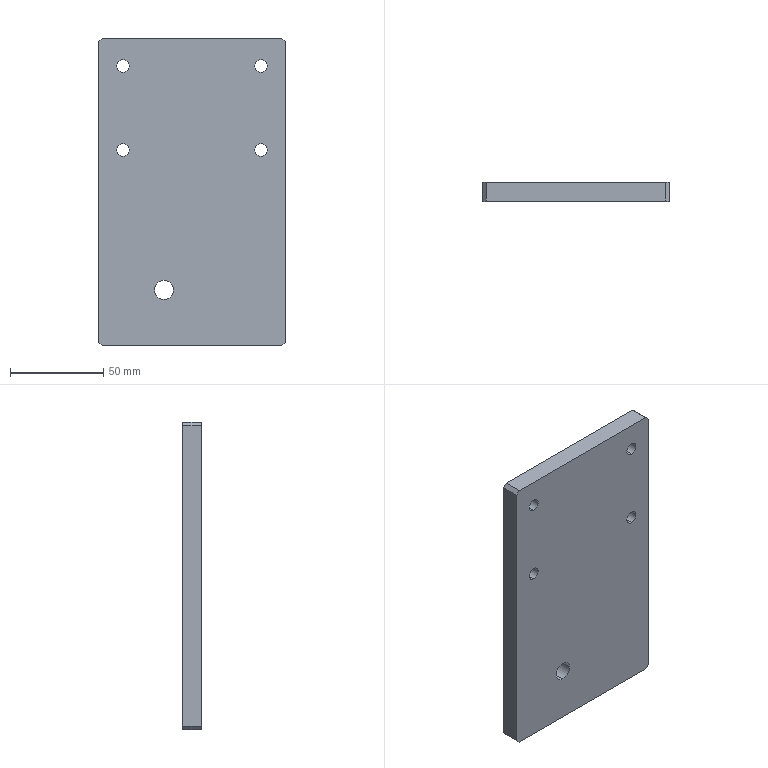Part | SolidWorks | features HoleWzd 3, 3DProfileFeature 2, Chamfer 1, Extrusion 1 | 1 solid | 20 faces | box 100 x 10 x 165 mm | volume 162650 mm3 | cylinder 10 | plane 10 | commonest cylinder face diameters 6.8 x8 10.2 x2
STEP:
#1=CARTESIAN_POINT('',(13.,0.,-56.6));
#2=VERTEX_POINT('',#1);
#3=CARTESIAN_POINT('',(13.,0.,-63.4));
#4=VERTEX_POINT('',#3);
#5=CARTESIAN_POINT('',(13.,0.,-60.));
#6=DIRECTION('',(0.,-1.,0.));
#7=DIRECTION('',(0.,0.,-1.));
#8=AXIS2_PLACEMENT_3D('',#5,#6,#7);
#9=CIRCLE('',#8,3.4);
#10=EDGE_CURVE('',#2,#4,#9,.T.);
#11=ORIENTED_EDGE('',*,*,#10,.T.);
#12=CARTESIAN_POINT('',(13.,10.,-63.4));
#13=VERTEX_POINT('',#12);
#14=CARTESIAN_POINT('',(13.,10.,-63.4));
#15=DIRECTION('',(0.,1.,0.));
#16=VECTOR('',#15,1000.);
#17=LINE('',#14,#16);
#18=EDGE_CURVE('',#4,#13,#17,.T.);
#19=ORIENTED_EDGE('',*,*,#18,.T.);
#20=CARTESIAN_POINT('',(13.,10.,-56.6));
#21=VERTEX_POINT('',#20);
#22=CARTESIAN_POINT('',(13.,10.,-60.));
#23=DIRECTION('',(0.,1.,0.));
#24=DIRECTION('',(0.,0.,1.));
#25=AXIS2_PLACEMENT_3D('',#22,#23,#24);
#26=CIRCLE('',#25,3.4);
#27=EDGE_CURVE('',#13,#21,#26,.T.);
#28=ORIENTED_EDGE('',*,*,#27,.T.);
#29=CARTESIAN_POINT('',(13.,10.,-56.6));
#30=DIRECTION('',(0.,1.,0.));
#31=VECTOR('',#30,1000.);
#32=LINE('',#29,#31);
#33=EDGE_CURVE('',#2,#21,#32,.T.);
#34=ORIENTED_EDGE('',*,*,#33,.F.);
#35=EDGE_LOOP('',(#11,#19,#28,#34));
#36=FACE_OUTER_BOUND('',#35,.T.);
#37=CARTESIAN_POINT('',(13.,10.,-60.));
#38=DIRECTION('',(0.,1.,0.));
#39=DIRECTION('',(0.,0.,1.));
#40=AXIS2_PLACEMENT_3D('',#37,#38,#39);
#41=CYLINDRICAL_SURFACE('',#40,3.4);
#42=ADVANCED_FACE('',(#36),#41,.F.);
#43=CARTESIAN_POINT('',(13.,0.,-11.6));
#44=VERTEX_POINT('',#43);
#45=CARTESIAN_POINT('',(13.,0.,-18.4));
#46=VERTEX_POINT('',#45);
#47=CARTESIAN_POINT('',(13.,0.,-15.));
#48=DIRECTION('',(0.,-1.,0.));
#49=DIRECTION('',(0.,0.,-1.));
#50=AXIS2_PLACEMENT_3D('',#47,#48,#49);
#51=CIRCLE('',#50,3.4);
#52=EDGE_CURVE('',#44,#46,#51,.T.);
#53=ORIENTED_EDGE('',*,*,#52,.T.);
#54=CARTESIAN_POINT('',(13.,10.,-18.4));
#55=VERTEX_POINT('',#54);
#56=CARTESIAN_POINT('',(13.,10.,-18.4));
#57=DIRECTION('',(0.,1.,0.));
#58=VECTOR('',#57,1000.);
#59=LINE('',#56,#58);
#60=EDGE_CURVE('',#46,#55,#59,.T.);
#61=ORIENTED_EDGE('',*,*,#60,.T.);
#62=CARTESIAN_POINT('',(13.,10.,-11.6));
#63=VERTEX_POINT('',#62);
#64=CARTESIAN_POINT('',(13.,10.,-15.));
#65=DIRECTION('',(0.,1.,0.));
#66=DIRECTION('',(0.,0.,1.));
#67=AXIS2_PLACEMENT_3D('',#64,#65,#66);
#68=CIRCLE('',#67,3.4);
#69=EDGE_CURVE('',#55,#63,#68,.T.);
#70=ORIENTED_EDGE('',*,*,#69,.T.);
#71=CARTESIAN_POINT('',(13.,10.,-11.6));
#72=DIRECTION('',(0.,1.,0.));
#73=VECTOR('',#72,1000.);
#74=LINE('',#71,#73);
#75=EDGE_CURVE('',#44,#63,#74,.T.);
#76=ORIENTED_EDGE('',*,*,#75,.F.);
#77=EDGE_LOOP('',(#53,#61,#70,#76));
#78=FACE_OUTER_BOUND('',#77,.T.);
#79=CARTESIAN_POINT('',(13.,10.,-15.));
#80=DIRECTION('',(0.,1.,0.));
#81=DIRECTION('',(0.,0.,1.));
#82=AXIS2_PLACEMENT_3D('',#79,#80,#81);
#83=CYLINDRICAL_SURFACE('',#82,3.4);
#84=ADVANCED_FACE('',(#78),#83,.F.);
#85=CARTESIAN_POINT('',(87.,0.,-11.6));
#86=VERTEX_POINT('',#85);
#87=CARTESIAN_POINT('',(87.,0.,-18.4));
#88=VERTEX_POINT('',#87);
#89=CARTESIAN_POINT('',(87.,0.,-15.));
#90=DIRECTION('',(0.,-1.,0.));
#91=DIRECTION('',(0.,0.,-1.));
#92=AXIS2_PLACEMENT_3D('',#89,#90,#91);
#93=CIRCLE('',#92,3.4);
#94=EDGE_CURVE('',#86,#88,#93,.T.);
#95=ORIENTED_EDGE('',*,*,#94,.T.);
#96=CARTESIAN_POINT('',(87.,10.,-18.4));
#97=VERTEX_POINT('',#96);
#98=CARTESIAN_POINT('',(87.,10.,-18.4));
#99=DIRECTION('',(0.,1.,0.));
#100=VECTOR('',#99,1000.);
#101=LINE('',#98,#100);
#102=EDGE_CURVE('',#88,#97,#101,.T.);
#103=ORIENTED_EDGE('',*,*,#102,.T.);
#104=CARTESIAN_POINT('',(87.,10.,-11.6));
#105=VERTEX_POINT('',#104);
#106=CARTESIAN_POINT('',(87.,10.,-15.));
#107=DIRECTION('',(0.,1.,0.));
#108=DIRECTION('',(0.,0.,1.));
#109=AXIS2_PLACEMENT_3D('',#106,#107,#108);
#110=CIRCLE('',#109,3.4);
#111=EDGE_CURVE('',#97,#105,#110,.T.);
#112=ORIENTED_EDGE('',*,*,#111,.T.);
#113=CARTESIAN_POINT('',(87.,10.,-11.6));
#114=DIRECTION('',(0.,1.,0.));
#115=VECTOR('',#114,1000.);
#116=LINE('',#113,#115);
#117=EDGE_CURVE('',#86,#105,#116,.T.);
#118=ORIENTED_EDGE('',*,*,#117,.F.);
#119=EDGE_LOOP('',(#95,#103,#112,#118));
#120=FACE_OUTER_BOUND('',#119,.T.);
#121=CARTESIAN_POINT('',(87.,10.,-15.));
#122=DIRECTION('',(0.,1.,0.));
#123=DIRECTION('',(0.,0.,1.));
#124=AXIS2_PLACEMENT_3D('',#121,#122,#123);
#125=CYLINDRICAL_SURFACE('',#124,3.4);
#126=ADVANCED_FACE('',(#120),#125,.F.);
#127=CARTESIAN_POINT('',(87.,0.,-56.6));
#128=VERTEX_POINT('',#127);
#129=CARTESIAN_POINT('',(87.,0.,-63.4));
#130=VERTEX_POINT('',#129);
#131=CARTESIAN_POINT('',(87.,0.,-60.));
#132=DIRECTION('',(0.,-1.,0.));
#133=DIRECTION('',(0.,0.,-1.));
#134=AXIS2_PLACEMENT_3D('',#131,#132,#133);
#135=CIRCLE('',#134,3.4);
#136=EDGE_CURVE('',#128,#130,#135,.T.);
#137=ORIENTED_EDGE('',*,*,#136,.T.);
#138=CARTESIAN_POINT('',(87.,10.,-63.4));
#139=VERTEX_POINT('',#138);
#140=CARTESIAN_POINT('',(87.,10.,-63.4));
#141=DIRECTION('',(0.,1.,0.));
#142=VECTOR('',#141,1000.);
#143=LINE('',#140,#142);
#144=EDGE_CURVE('',#130,#139,#143,.T.);
#145=ORIENTED_EDGE('',*,*,#144,.T.);
#146=CARTESIAN_POINT('',(87.,10.,-56.6));
#147=VERTEX_POINT('',#146);
#148=CARTESIAN_POINT('',(87.,10.,-60.));
#149=DIRECTION('',(0.,1.,0.));
#150=DIRECTION('',(0.,0.,1.));
#151=AXIS2_PLACEMENT_3D('',#148,#149,#150);
#152=CIRCLE('',#151,3.4);
#153=EDGE_CURVE('',#139,#147,#152,.T.);
#154=ORIENTED_EDGE('',*,*,#153,.T.);
#155=CARTESIAN_POINT('',(87.,10.,-56.6));
#156=DIRECTION('',(0.,1.,0.));
#157=VECTOR('',#156,1000.);
#158=LINE('',#155,#157);
#159=EDGE_CURVE('',#128,#147,#158,.T.);
#160=ORIENTED_EDGE('',*,*,#159,.F.);
#161=EDGE_LOOP('',(#137,#145,#154,#160));
#162=FACE_OUTER_BOUND('',#161,.T.);
#163=CARTESIAN_POINT('',(87.,10.,-60.));
#164=DIRECTION('',(0.,1.,0.));
#165=DIRECTION('',(0.,0.,1.));
#166=AXIS2_PLACEMENT_3D('',#163,#164,#165);
#167=CYLINDRICAL_SURFACE('',#166,3.4);
#168=ADVANCED_FACE('',(#162),#167,.F.);
#169=CARTESIAN_POINT('',(35.,0.,-129.9));
#170=VERTEX_POINT('',#169);
#171=CARTESIAN_POINT('',(35.,0.,-140.1));
#172=VERTEX_POINT('',#171);
#173=CARTESIAN_POINT('',(35.,0.,-135.));
#174=DIRECTION('',(0.,-1.,0.));
#175=DIRECTION('',(0.,0.,-1.));
#176=AXIS2_PLACEMENT_3D('',#173,#174,#175);
#177=CIRCLE('',#176,5.1);
#178=EDGE_CURVE('',#170,#172,#177,.T.);
#179=ORIENTED_EDGE('',*,*,#178,.T.);
#180=CARTESIAN_POINT('',(35.,10.,-140.1));
#181=VERTEX_POINT('',#180);
#182=CARTESIAN_POINT('',(35.,10.,-140.1));
#183=DIRECTION('',(0.,1.,0.));
#184=VECTOR('',#183,1000.);
#185=LINE('',#182,#184);
#186=EDGE_CURVE('',#172,#181,#185,.T.);
#187=ORIENTED_EDGE('',*,*,#186,.T.);
#188=CARTESIAN_POINT('',(35.,10.,-129.9));
#189=VERTEX_POINT('',#188);
#190=CARTESIAN_POINT('',(35.,10.,-135.));
#191=DIRECTION('',(0.,1.,0.));
#192=DIRECTION('',(0.,0.,1.));
#193=AXIS2_PLACEMENT_3D('',#190,#191,#192);
#194=CIRCLE('',#193,5.1);
#195=EDGE_CURVE('',#181,#189,#194,.T.);
#196=ORIENTED_EDGE('',*,*,#195,.T.);
#197=CARTESIAN_POINT('',(35.,10.,-129.9));
#198=DIRECTION('',(0.,1.,0.));
#199=VECTOR('',#198,1000.);
#200=LINE('',#197,#199);
#201=EDGE_CURVE('',#170,#189,#200,.T.);
#202=ORIENTED_EDGE('',*,*,#201,.F.);
#203=EDGE_LOOP('',(#179,#187,#196,#202));
#204=FACE_OUTER_BOUND('',#203,.T.);
#205=CARTESIAN_POINT('',(35.,10.,-135.));
#206=DIRECTION('',(0.,1.,0.));
#207=DIRECTION('',(0.,0.,1.));
#208=AXIS2_PLACEMENT_3D('',#205,#206,#207);
#209=CYLINDRICAL_SURFACE('',#208,5.1);
#210=ADVANCED_FACE('',(#204),#209,.F.);
#211=CARTESIAN_POINT('',(13.,10.,-15.));
#212=DIRECTION('',(0.,1.,0.));
#213=DIRECTION('',(0.,0.,1.));
#214=AXIS2_PLACEMENT_3D('',#211,#212,#213);
#215=CIRCLE('',#214,3.4);
#216=EDGE_CURVE('',#63,#55,#215,.T.);
#217=ORIENTED_EDGE('',*,*,#216,.F.);
#218=ORIENTED_EDGE('',*,*,#69,.F.);
#219=EDGE_LOOP('',(#217,#218));
#220=FACE_BOUND('',#219,.T.);
#221=CARTESIAN_POINT('',(87.,10.,-15.));
#222=DIRECTION('',(0.,1.,0.));
#223=DIRECTION('',(0.,0.,1.));
#224=AXIS2_PLACEMENT_3D('',#221,#222,#223);
#225=CIRCLE('',#224,3.4);
#226=EDGE_CURVE('',#105,#97,#225,.T.);
#227=ORIENTED_EDGE('',*,*,#226,.F.);
#228=ORIENTED_EDGE('',*,*,#111,.F.);
#229=EDGE_LOOP('',(#227,#228));
#230=FACE_BOUND('',#229,.T.);
#231=CARTESIAN_POINT('',(87.,10.,-60.));
#232=DIRECTION('',(0.,1.,0.));
#233=DIRECTION('',(0.,0.,1.));
#234=AXIS2_PLACEMENT_3D('',#231,#232,#233);
#235=CIRCLE('',#234,3.4);
#236=EDGE_CURVE('',#147,#139,#235,.T.);
#237=ORIENTED_EDGE('',*,*,#236,.F.);
#238=ORIENTED_EDGE('',*,*,#153,.F.);
#239=EDGE_LOOP('',(#237,#238));
#240=FACE_BOUND('',#239,.T.);
#241=CARTESIAN_POINT('',(35.,10.,-135.));
#242=DIRECTION('',(0.,1.,0.));
#243=DIRECTION('',(0.,0.,1.));
#244=AXIS2_PLACEMENT_3D('',#241,#242,#243);
#245=CIRCLE('',#244,5.1);
#246=EDGE_CURVE('',#189,#181,#245,.T.);
#247=ORIENTED_EDGE('',*,*,#246,.F.);
#248=ORIENTED_EDGE('',*,*,#195,.F.);
#249=EDGE_LOOP('',(#247,#248));
#250=FACE_BOUND('',#249,.T.);
#251=CARTESIAN_POINT('',(2.,10.,0.));
#252=VERTEX_POINT('',#251);
#253=CARTESIAN_POINT('',(98.,10.,0.));
#254=VERTEX_POINT('',#253);
#255=CARTESIAN_POINT('',(0.,10.,0.));
#256=DIRECTION('',(1.,0.,0.));
#257=VECTOR('',#256,1000.);
#258=LINE('',#255,#257);
#259=EDGE_CURVE('',#252,#254,#258,.T.);
#260=ORIENTED_EDGE('',*,*,#259,.T.);
#261=CARTESIAN_POINT('',(100.,10.,-2.));
#262=VERTEX_POINT('',#261);
#263=CARTESIAN_POINT('',(100.,10.,-2.));
#264=DIRECTION('',(0.7071,0.,-0.7071));
#265=VECTOR('',#264,1000.);
#266=LINE('',#263,#265);
#267=EDGE_CURVE('',#254,#262,#266,.T.);
#268=ORIENTED_EDGE('',*,*,#267,.T.);
#269=CARTESIAN_POINT('',(100.,10.,-163.));
#270=VERTEX_POINT('',#269);
#271=CARTESIAN_POINT('',(100.,10.,0.));
#272=DIRECTION('',(0.,0.,-1.));
#273=VECTOR('',#272,1000.);
#274=LINE('',#271,#273);
#275=EDGE_CURVE('',#262,#270,#274,.T.);
#276=ORIENTED_EDGE('',*,*,#275,.T.);
#277=CARTESIAN_POINT('',(98.,10.,-165.));
#278=VERTEX_POINT('',#277);
#279=CARTESIAN_POINT('',(98.,10.,-165.));
#280=DIRECTION('',(-0.7071,0.,-0.7071));
#281=VECTOR('',#280,1000.);
#282=LINE('',#279,#281);
#283=EDGE_CURVE('',#270,#278,#282,.T.);
#284=ORIENTED_EDGE('',*,*,#283,.T.);
#285=CARTESIAN_POINT('',(2.,10.,-165.));
#286=VERTEX_POINT('',#285);
#287=CARTESIAN_POINT('',(0.,10.,-165.));
#288=DIRECTION('',(-1.,0.,0.));
#289=VECTOR('',#288,1000.);
#290=LINE('',#287,#289);
#291=EDGE_CURVE('',#278,#286,#290,.T.);
#292=ORIENTED_EDGE('',*,*,#291,.T.);
#293=CARTESIAN_POINT('',(0.,10.,-163.));
#294=VERTEX_POINT('',#293);
#295=CARTESIAN_POINT('',(0.,10.,-163.));
#296=DIRECTION('',(-0.7071,0.,0.7071));
#297=VECTOR('',#296,1000.);
#298=LINE('',#295,#297);
#299=EDGE_CURVE('',#286,#294,#298,.T.);
#300=ORIENTED_EDGE('',*,*,#299,.T.);
#301=CARTESIAN_POINT('',(0.,10.,-2.));
#302=VERTEX_POINT('',#301);
#303=CARTESIAN_POINT('',(0.,10.,0.));
#304=DIRECTION('',(0.,0.,1.));
#305=VECTOR('',#304,1000.);
#306=LINE('',#303,#305);
#307=EDGE_CURVE('',#294,#302,#306,.T.);
#308=ORIENTED_EDGE('',*,*,#307,.T.);
#309=CARTESIAN_POINT('',(2.,10.,0.));
#310=DIRECTION('',(0.7071,0.,0.7071));
#311=VECTOR('',#310,1000.);
#312=LINE('',#309,#311);
#313=EDGE_CURVE('',#302,#252,#312,.T.);
#314=ORIENTED_EDGE('',*,*,#313,.T.);
#315=EDGE_LOOP('',(#260,#268,#276,#284,#292,#300,#308,#314));
#316=FACE_OUTER_BOUND('',#315,.T.);
#317=CARTESIAN_POINT('',(13.,10.,-60.));
#318=DIRECTION('',(0.,1.,0.));
#319=DIRECTION('',(0.,0.,1.));
#320=AXIS2_PLACEMENT_3D('',#317,#318,#319);
#321=CIRCLE('',#320,3.4);
#322=EDGE_CURVE('',#21,#13,#321,.T.);
#323=ORIENTED_EDGE('',*,*,#322,.F.);
#324=ORIENTED_EDGE('',*,*,#27,.F.);
#325=EDGE_LOOP('',(#323,#324));
#326=FACE_BOUND('',#325,.T.);
#327=CARTESIAN_POINT('',(0.,10.,0.));
#328=DIRECTION('',(0.,-1.,0.));
#329=DIRECTION('',(0.,0.,-1.));
#330=AXIS2_PLACEMENT_3D('',#327,#328,#329);
#331=PLANE('',#330);
#332=ADVANCED_FACE('',(#220,#230,#240,#250,#316,#326),#331,.F.);
#333=CARTESIAN_POINT('',(0.,0.,-163.));
#334=VERTEX_POINT('',#333);
#335=CARTESIAN_POINT('',(0.,0.,-2.));
#336=VERTEX_POINT('',#335);
#337=CARTESIAN_POINT('',(0.,0.,0.));
#338=DIRECTION('',(0.,0.,1.));
#339=VECTOR('',#338,1000.);
#340=LINE('',#337,#339);
#341=EDGE_CURVE('',#334,#336,#340,.T.);
#342=ORIENTED_EDGE('',*,*,#341,.T.);
#343=CARTESIAN_POINT('',(0.,10.,-2.));
#344=DIRECTION('',(0.,1.,0.));
#345=VECTOR('',#344,1000.);
#346=LINE('',#343,#345);
#347=EDGE_CURVE('',#336,#302,#346,.T.);
#348=ORIENTED_EDGE('',*,*,#347,.T.);
#349=ORIENTED_EDGE('',*,*,#307,.F.);
#350=CARTESIAN_POINT('',(0.,10.,-163.));
#351=DIRECTION('',(0.,-1.,0.));
#352=VECTOR('',#351,1000.);
#353=LINE('',#350,#352);
#354=EDGE_CURVE('',#294,#334,#353,.T.);
#355=ORIENTED_EDGE('',*,*,#354,.T.);
#356=EDGE_LOOP('',(#342,#348,#349,#355));
#357=FACE_OUTER_BOUND('',#356,.T.);
#358=CARTESIAN_POINT('',(0.,10.,0.));
#359=DIRECTION('',(1.,0.,0.));
#360=DIRECTION('',(0.,0.,-1.));
#361=AXIS2_PLACEMENT_3D('',#358,#359,#360);
#362=PLANE('',#361);
#363=ADVANCED_FACE('',(#357),#362,.F.);
#364=CARTESIAN_POINT('',(2.,0.,0.));
#365=VERTEX_POINT('',#364);
#366=CARTESIAN_POINT('',(98.,0.,0.));
#367=VERTEX_POINT('',#366);
#368=CARTESIAN_POINT('',(0.,0.,0.));
#369=DIRECTION('',(1.,0.,0.));
#370=VECTOR('',#369,1000.);
#371=LINE('',#368,#370);
#372=EDGE_CURVE('',#365,#367,#371,.T.);
#373=ORIENTED_EDGE('',*,*,#372,.T.);
#374=CARTESIAN_POINT('',(98.,10.,0.));
#375=DIRECTION('',(0.,1.,0.));
#376=VECTOR('',#375,1000.);
#377=LINE('',#374,#376);
#378=EDGE_CURVE('',#367,#254,#377,.T.);
#379=ORIENTED_EDGE('',*,*,#378,.T.);
#380=ORIENTED_EDGE('',*,*,#259,.F.);
#381=CARTESIAN_POINT('',(2.,10.,0.));
#382=DIRECTION('',(0.,-1.,0.));
#383=VECTOR('',#382,1000.);
#384=LINE('',#381,#383);
#385=EDGE_CURVE('',#252,#365,#384,.T.);
#386=ORIENTED_EDGE('',*,*,#385,.T.);
#387=EDGE_LOOP('',(#373,#379,#380,#386));
#388=FACE_OUTER_BOUND('',#387,.T.);
#389=CARTESIAN_POINT('',(0.,10.,0.));
#390=DIRECTION('',(0.,0.,-1.));
#391=DIRECTION('',(-1.,0.,0.));
#392=AXIS2_PLACEMENT_3D('',#389,#390,#391);
#393=PLANE('',#392);
#394=ADVANCED_FACE('',(#388),#393,.F.);
#395=ORIENTED_EDGE('',*,*,#275,.F.);
#396=CARTESIAN_POINT('',(100.,0.,-2.));
#397=VERTEX_POINT('',#396);
#398=CARTESIAN_POINT('',(100.,10.,-2.));
#399=DIRECTION('',(0.,-1.,0.));
#400=VECTOR('',#399,1000.);
#401=LINE('',#398,#400);
#402=EDGE_CURVE('',#262,#397,#401,.T.);
#403=ORIENTED_EDGE('',*,*,#402,.T.);
#404=CARTESIAN_POINT('',(100.,0.,-163.));
#405=VERTEX_POINT('',#404);
#406=CARTESIAN_POINT('',(100.,0.,0.));
#407=DIRECTION('',(0.,0.,-1.));
#408=VECTOR('',#407,1000.);
#409=LINE('',#406,#408);
#410=EDGE_CURVE('',#397,#405,#409,.T.);
#411=ORIENTED_EDGE('',*,*,#410,.T.);
#412=CARTESIAN_POINT('',(100.,10.,-163.));
#413=DIRECTION('',(0.,1.,0.));
#414=VECTOR('',#413,1000.);
#415=LINE('',#412,#414);
#416=EDGE_CURVE('',#405,#270,#415,.T.);
#417=ORIENTED_EDGE('',*,*,#416,.T.);
#418=EDGE_LOOP('',(#395,#403,#411,#417));
#419=FACE_OUTER_BOUND('',#418,.T.);
#420=CARTESIAN_POINT('',(100.,10.,0.));
#421=DIRECTION('',(-1.,0.,0.));
#422=DIRECTION('',(0.,0.,1.));
#423=AXIS2_PLACEMENT_3D('',#420,#421,#422);
#424=PLANE('',#423);
#425=ADVANCED_FACE('',(#419),#424,.F.);
#426=ORIENTED_EDGE('',*,*,#291,.F.);
#427=CARTESIAN_POINT('',(98.,0.,-165.));
#428=VERTEX_POINT('',#427);
#429=CARTESIAN_POINT('',(98.,10.,-165.));
#430=DIRECTION('',(0.,-1.,0.));
#431=VECTOR('',#430,1000.);
#432=LINE('',#429,#431);
#433=EDGE_CURVE('',#278,#428,#432,.T.);
#434=ORIENTED_EDGE('',*,*,#433,.T.);
#435=CARTESIAN_POINT('',(2.,0.,-165.));
#436=VERTEX_POINT('',#435);
#437=CARTESIAN_POINT('',(0.,0.,-165.));
#438=DIRECTION('',(-1.,0.,0.));
#439=VECTOR('',#438,1000.);
#440=LINE('',#437,#439);
#441=EDGE_CURVE('',#428,#436,#440,.T.);
#442=ORIENTED_EDGE('',*,*,#441,.T.);
#443=CARTESIAN_POINT('',(2.,10.,-165.));
#444=DIRECTION('',(0.,1.,0.));
#445=VECTOR('',#444,1000.);
#446=LINE('',#443,#445);
#447=EDGE_CURVE('',#436,#286,#446,.T.);
#448=ORIENTED_EDGE('',*,*,#447,.T.);
#449=EDGE_LOOP('',(#426,#434,#442,#448));
#450=FACE_OUTER_BOUND('',#449,.T.);
#451=CARTESIAN_POINT('',(0.,10.,-165.));
#452=DIRECTION('',(0.,0.,1.));
#453=DIRECTION('',(1.,0.,0.));
#454=AXIS2_PLACEMENT_3D('',#451,#452,#453);
#455=PLANE('',#454);
#456=ADVANCED_FACE('',(#450),#455,.F.);
#457=ORIENTED_EDGE('',*,*,#10,.F.);
#458=CARTESIAN_POINT('',(13.,0.,-60.));
#459=DIRECTION('',(0.,-1.,0.));
#460=DIRECTION('',(0.,0.,-1.));
#461=AXIS2_PLACEMENT_3D('',#458,#459,#460);
#462=CIRCLE('',#461,3.4);
#463=EDGE_CURVE('',#4,#2,#462,.T.);
#464=ORIENTED_EDGE('',*,*,#463,.F.);
#465=EDGE_LOOP('',(#457,#464));
#466=FACE_BOUND('',#465,.T.);
#467=ORIENTED_EDGE('',*,*,#52,.F.);
#468=CARTESIAN_POINT('',(13.,0.,-15.));
#469=DIRECTION('',(0.,-1.,0.));
#470=DIRECTION('',(0.,0.,-1.));
#471=AXIS2_PLACEMENT_3D('',#468,#469,#470);
#472=CIRCLE('',#471,3.4);
#473=EDGE_CURVE('',#46,#44,#472,.T.);
#474=ORIENTED_EDGE('',*,*,#473,.F.);
#475=EDGE_LOOP('',(#467,#474));
#476=FACE_BOUND('',#475,.T.);
#477=ORIENTED_EDGE('',*,*,#94,.F.);
#478=CARTESIAN_POINT('',(87.,0.,-15.));
#479=DIRECTION('',(0.,-1.,0.));
#480=DIRECTION('',(0.,0.,-1.));
#481=AXIS2_PLACEMENT_3D('',#478,#479,#480);
#482=CIRCLE('',#481,3.4);
#483=EDGE_CURVE('',#88,#86,#482,.T.);
#484=ORIENTED_EDGE('',*,*,#483,.F.);
#485=EDGE_LOOP('',(#477,#484));
#486=FACE_BOUND('',#485,.T.);
#487=ORIENTED_EDGE('',*,*,#136,.F.);
#488=CARTESIAN_POINT('',(87.,0.,-60.));
#489=DIRECTION('',(0.,-1.,0.));
#490=DIRECTION('',(0.,0.,-1.));
#491=AXIS2_PLACEMENT_3D('',#488,#489,#490);
#492=CIRCLE('',#491,3.4);
#493=EDGE_CURVE('',#130,#128,#492,.T.);
#494=ORIENTED_EDGE('',*,*,#493,.F.);
#495=EDGE_LOOP('',(#487,#494));
#496=FACE_BOUND('',#495,.T.);
#497=ORIENTED_EDGE('',*,*,#178,.F.);
#498=CARTESIAN_POINT('',(35.,0.,-135.));
#499=DIRECTION('',(0.,-1.,0.));
#500=DIRECTION('',(0.,0.,-1.));
#501=AXIS2_PLACEMENT_3D('',#498,#499,#500);
#502=CIRCLE('',#501,5.1);
#503=EDGE_CURVE('',#172,#170,#502,.T.);
#504=ORIENTED_EDGE('',*,*,#503,.F.);
#505=EDGE_LOOP('',(#497,#504));
#506=FACE_BOUND('',#505,.T.);
#507=ORIENTED_EDGE('',*,*,#410,.F.);
#508=CARTESIAN_POINT('',(49.,0.,49.));
#509=DIRECTION('',(-0.7071,0.,0.7071));
#510=VECTOR('',#509,1000.);
#511=LINE('',#508,#510);
#512=EDGE_CURVE('',#397,#367,#511,.T.);
#513=ORIENTED_EDGE('',*,*,#512,.T.);
#514=ORIENTED_EDGE('',*,*,#372,.F.);
#515=CARTESIAN_POINT('',(1.,0.,-1.));
#516=DIRECTION('',(-0.7071,0.,-0.7071));
#517=VECTOR('',#516,1000.);
#518=LINE('',#515,#517);
#519=EDGE_CURVE('',#365,#336,#518,.T.);
#520=ORIENTED_EDGE('',*,*,#519,.T.);
#521=ORIENTED_EDGE('',*,*,#341,.F.);
#522=CARTESIAN_POINT('',(-81.5,0.,-81.5));
#523=DIRECTION('',(0.7071,0.,-0.7071));
#524=VECTOR('',#523,1000.);
#525=LINE('',#522,#524);
#526=EDGE_CURVE('',#334,#436,#525,.T.);
#527=ORIENTED_EDGE('',*,*,#526,.T.);
#528=ORIENTED_EDGE('',*,*,#441,.F.);
#529=CARTESIAN_POINT('',(131.5,0.,-131.5));
#530=DIRECTION('',(0.7071,0.,0.7071));
#531=VECTOR('',#530,1000.);
#532=LINE('',#529,#531);
#533=EDGE_CURVE('',#428,#405,#532,.T.);
#534=ORIENTED_EDGE('',*,*,#533,.T.);
#535=EDGE_LOOP('',(#507,#513,#514,#520,#521,#527,#528,#534));
#536=FACE_OUTER_BOUND('',#535,.T.);
#537=CARTESIAN_POINT('',(0.,0.,0.));
#538=DIRECTION('',(0.,-1.,0.));
#539=DIRECTION('',(0.,0.,-1.));
#540=AXIS2_PLACEMENT_3D('',#537,#538,#539);
#541=PLANE('',#540);
#542=ADVANCED_FACE('',(#466,#476,#486,#496,#506,#536),#541,.T.);
#543=ORIENTED_EDGE('',*,*,#267,.F.);
#544=ORIENTED_EDGE('',*,*,#378,.F.);
#545=ORIENTED_EDGE('',*,*,#512,.F.);
#546=ORIENTED_EDGE('',*,*,#402,.F.);
#547=EDGE_LOOP('',(#543,#544,#545,#546));
#548=FACE_OUTER_BOUND('',#547,.T.);
#549=CARTESIAN_POINT('',(100.,10.,-2.));
#550=DIRECTION('',(-0.7071,0.,-0.7071));
#551=DIRECTION('',(0.,-1.,0.));
#552=AXIS2_PLACEMENT_3D('',#549,#550,#551);
#553=PLANE('',#552);
#554=ADVANCED_FACE('',(#548),#553,.F.);
#555=ORIENTED_EDGE('',*,*,#313,.F.);
#556=ORIENTED_EDGE('',*,*,#347,.F.);
#557=ORIENTED_EDGE('',*,*,#519,.F.);
#558=ORIENTED_EDGE('',*,*,#385,.F.);
#559=EDGE_LOOP('',(#555,#556,#557,#558));
#560=FACE_OUTER_BOUND('',#559,.T.);
#561=CARTESIAN_POINT('',(2.,10.,0.));
#562=DIRECTION('',(0.7071,0.,-0.7071));
#563=DIRECTION('',(0.,-1.,0.));
#564=AXIS2_PLACEMENT_3D('',#561,#562,#563);
#565=PLANE('',#564);
#566=ADVANCED_FACE('',(#560),#565,.F.);
#567=ORIENTED_EDGE('',*,*,#283,.F.);
#568=ORIENTED_EDGE('',*,*,#416,.F.);
#569=ORIENTED_EDGE('',*,*,#533,.F.);
#570=ORIENTED_EDGE('',*,*,#433,.F.);
#571=EDGE_LOOP('',(#567,#568,#569,#570));
#572=FACE_OUTER_BOUND('',#571,.T.);
#573=CARTESIAN_POINT('',(98.,10.,-165.));
#574=DIRECTION('',(-0.7071,0.,0.7071));
#575=DIRECTION('',(0.,-1.,0.));
#576=AXIS2_PLACEMENT_3D('',#573,#574,#575);
#577=PLANE('',#576);
#578=ADVANCED_FACE('',(#572),#577,.F.);
#579=ORIENTED_EDGE('',*,*,#299,.F.);
#580=ORIENTED_EDGE('',*,*,#447,.F.);
#581=ORIENTED_EDGE('',*,*,#526,.F.);
#582=ORIENTED_EDGE('',*,*,#354,.F.);
#583=EDGE_LOOP('',(#579,#580,#581,#582));
#584=FACE_OUTER_BOUND('',#583,.T.);
#585=CARTESIAN_POINT('',(0.,10.,-163.));
#586=DIRECTION('',(0.7071,0.,0.7071));
#587=DIRECTION('',(0.,-1.,0.));
#588=AXIS2_PLACEMENT_3D('',#585,#586,#587);
#589=PLANE('',#588);
#590=ADVANCED_FACE('',(#584),#589,.F.);
#591=ORIENTED_EDGE('',*,*,#186,.F.);
#592=ORIENTED_EDGE('',*,*,#503,.T.);
#593=ORIENTED_EDGE('',*,*,#201,.T.);
#594=ORIENTED_EDGE('',*,*,#246,.T.);
#595=EDGE_LOOP('',(#591,#592,#593,#594));
#596=FACE_OUTER_BOUND('',#595,.T.);
#597=CARTESIAN_POINT('',(35.,10.,-135.));
#598=DIRECTION('',(0.,1.,0.));
#599=DIRECTION('',(0.,0.,1.));
#600=AXIS2_PLACEMENT_3D('',#597,#598,#599);
#601=CYLINDRICAL_SURFACE('',#600,5.1);
#602=ADVANCED_FACE('',(#596),#601,.F.);
#603=ORIENTED_EDGE('',*,*,#144,.F.);
#604=ORIENTED_EDGE('',*,*,#493,.T.);
#605=ORIENTED_EDGE('',*,*,#159,.T.);
#606=ORIENTED_EDGE('',*,*,#236,.T.);
#607=EDGE_LOOP('',(#603,#604,#605,#606));
#608=FACE_OUTER_BOUND('',#607,.T.);
#609=CARTESIAN_POINT('',(87.,10.,-60.));
#610=DIRECTION('',(0.,1.,0.));
#611=DIRECTION('',(0.,0.,1.));
#612=AXIS2_PLACEMENT_3D('',#609,#610,#611);
#613=CYLINDRICAL_SURFACE('',#612,3.4);
#614=ADVANCED_FACE('',(#608),#613,.F.);
#615=ORIENTED_EDGE('',*,*,#102,.F.);
#616=ORIENTED_EDGE('',*,*,#483,.T.);
#617=ORIENTED_EDGE('',*,*,#117,.T.);
#618=ORIENTED_EDGE('',*,*,#226,.T.);
#619=EDGE_LOOP('',(#615,#616,#617,#618));
#620=FACE_OUTER_BOUND('',#619,.T.);
#621=CARTESIAN_POINT('',(87.,10.,-15.));
#622=DIRECTION('',(0.,1.,0.));
#623=DIRECTION('',(0.,0.,1.));
#624=AXIS2_PLACEMENT_3D('',#621,#622,#623);
#625=CYLINDRICAL_SURFACE('',#624,3.4);
#626=ADVANCED_FACE('',(#620),#625,.F.);
#627=ORIENTED_EDGE('',*,*,#60,.F.);
#628=ORIENTED_EDGE('',*,*,#473,.T.);
#629=ORIENTED_EDGE('',*,*,#75,.T.);
#630=ORIENTED_EDGE('',*,*,#216,.T.);
#631=EDGE_LOOP('',(#627,#628,#629,#630));
#632=FACE_OUTER_BOUND('',#631,.T.);
#633=CARTESIAN_POINT('',(13.,10.,-15.));
#634=DIRECTION('',(0.,1.,0.));
#635=DIRECTION('',(0.,0.,1.));
#636=AXIS2_PLACEMENT_3D('',#633,#634,#635);
#637=CYLINDRICAL_SURFACE('',#636,3.4);
#638=ADVANCED_FACE('',(#632),#637,.F.);
#639=ORIENTED_EDGE('',*,*,#18,.F.);
#640=ORIENTED_EDGE('',*,*,#463,.T.);
#641=ORIENTED_EDGE('',*,*,#33,.T.);
#642=ORIENTED_EDGE('',*,*,#322,.T.);
#643=EDGE_LOOP('',(#639,#640,#641,#642));
#644=FACE_OUTER_BOUND('',#643,.T.);
#645=CARTESIAN_POINT('',(13.,10.,-60.));
#646=DIRECTION('',(0.,1.,0.));
#647=DIRECTION('',(0.,0.,1.));
#648=AXIS2_PLACEMENT_3D('',#645,#646,#647);
#649=CYLINDRICAL_SURFACE('',#648,3.4);
#650=ADVANCED_FACE('',(#644),#649,.F.);
#651=CLOSED_SHELL('',(#42,#84,#126,#168,#210,#332,#363,#394,#425,#456,#542,#554,#566,#578,#590,#602,#614,#626,#638,#650));
#652=MANIFOLD_SOLID_BREP('',#651);
#653=CARTESIAN_POINT('',(0.,0.,0.));
#654=DIRECTION('',(0.,0.,1.));
#655=DIRECTION('',(1.,0.,0.));
#656=AXIS2_PLACEMENT_3D('',#653,#654,#655);
#657=(LENGTH_UNIT()NAMED_UNIT(*)SI_UNIT(.MILLI.,.METRE.));
#658=UNCERTAINTY_MEASURE_WITH_UNIT(LENGTH_MEASURE(0.00001),#657,'','');
#659=(NAMED_UNIT(*)PLANE_ANGLE_UNIT()SI_UNIT($,.RADIAN.));
#660=(NAMED_UNIT(*)SI_UNIT($,.STERADIAN.)SOLID_ANGLE_UNIT());
#661=(GEOMETRIC_REPRESENTATION_CONTEXT(3)GLOBAL_UNCERTAINTY_ASSIGNED_CONTEXT((#658))GLOBAL_UNIT_ASSIGNED_CONTEXT((#657,#659,#660))REPRESENTATION_CONTEXT('',''));
#662=ADVANCED_BREP_SHAPE_REPRESENTATION('',(#652,#656),#661);